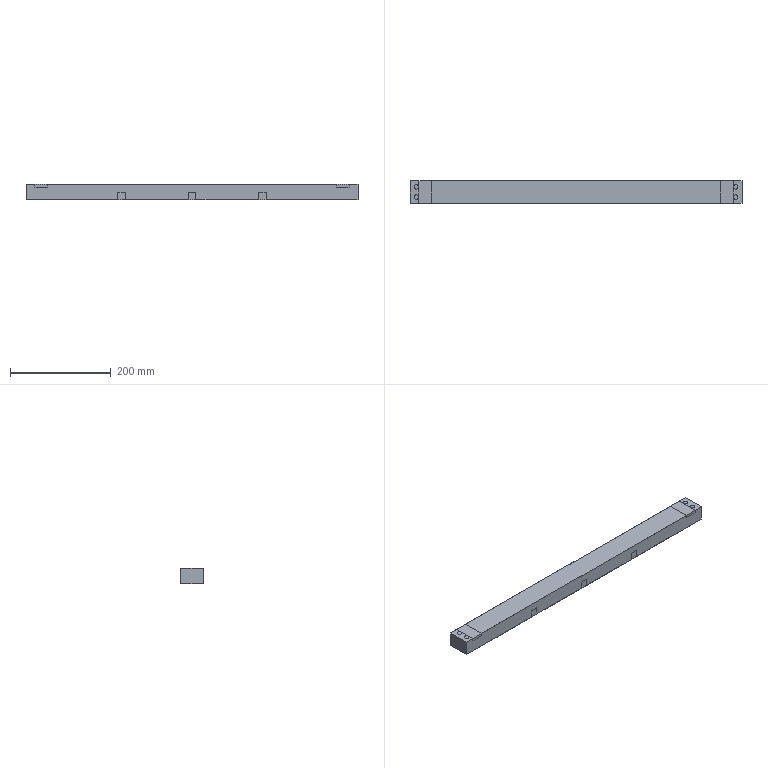Part | 2 solids | 70 faces | box 659.9 x 45 x 30 mm | volume 1746245 mm3 | cylinder 39 | plane 31 | commonest cylinder face diameters 9 x16 14 x16 8 x4 32 x3